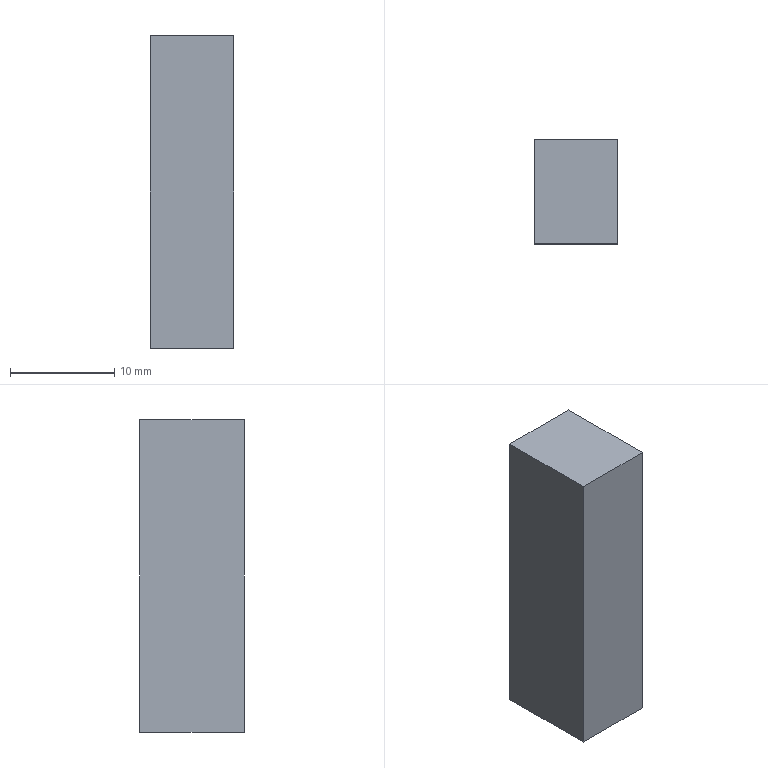Part | SolidWorks | features Extrusion 1 | 1 solid | 6 faces | box 8 x 10 x 30 mm | volume 2400 mm3 | plane 6
STEP:
#1=CARTESIAN_POINT('',(4.,0.,15.));
#2=VERTEX_POINT('',#1);
#3=CARTESIAN_POINT('',(4.,0.,-15.));
#4=VERTEX_POINT('',#3);
#5=CARTESIAN_POINT('',(4.,0.,-15.));
#6=DIRECTION('',(0.,0.,-1.));
#7=VECTOR('',#6,1000.);
#8=LINE('',#5,#7);
#9=EDGE_CURVE('',#2,#4,#8,.T.);
#10=ORIENTED_EDGE('',*,*,#9,.T.);
#11=CARTESIAN_POINT('',(4.,10.,-15.));
#12=VERTEX_POINT('',#11);
#13=CARTESIAN_POINT('',(4.,10.,-15.));
#14=DIRECTION('',(0.,-1.,0.));
#15=VECTOR('',#14,1000.);
#16=LINE('',#13,#15);
#17=EDGE_CURVE('',#12,#4,#16,.T.);
#18=ORIENTED_EDGE('',*,*,#17,.F.);
#19=CARTESIAN_POINT('',(4.,10.,15.));
#20=VERTEX_POINT('',#19);
#21=CARTESIAN_POINT('',(4.,10.,-15.));
#22=DIRECTION('',(0.,0.,-1.));
#23=VECTOR('',#22,1000.);
#24=LINE('',#21,#23);
#25=EDGE_CURVE('',#20,#12,#24,.T.);
#26=ORIENTED_EDGE('',*,*,#25,.F.);
#27=CARTESIAN_POINT('',(4.,10.,15.));
#28=DIRECTION('',(0.,-1.,0.));
#29=VECTOR('',#28,1000.);
#30=LINE('',#27,#29);
#31=EDGE_CURVE('',#20,#2,#30,.T.);
#32=ORIENTED_EDGE('',*,*,#31,.T.);
#33=EDGE_LOOP('',(#10,#18,#26,#32));
#34=FACE_OUTER_BOUND('',#33,.T.);
#35=CARTESIAN_POINT('',(4.,10.,-15.));
#36=DIRECTION('',(-1.,0.,0.));
#37=DIRECTION('',(0.,0.,1.));
#38=AXIS2_PLACEMENT_3D('',#35,#36,#37);
#39=PLANE('',#38);
#40=ADVANCED_FACE('',(#34),#39,.F.);
#41=CARTESIAN_POINT('',(-4.,0.,-15.));
#42=VERTEX_POINT('',#41);
#43=CARTESIAN_POINT('',(-4.,0.,-15.));
#44=DIRECTION('',(-1.,0.,0.));
#45=VECTOR('',#44,1000.);
#46=LINE('',#43,#45);
#47=EDGE_CURVE('',#4,#42,#46,.T.);
#48=ORIENTED_EDGE('',*,*,#47,.T.);
#49=CARTESIAN_POINT('',(-4.,10.,-15.));
#50=VERTEX_POINT('',#49);
#51=CARTESIAN_POINT('',(-4.,10.,-15.));
#52=DIRECTION('',(0.,-1.,0.));
#53=VECTOR('',#52,1000.);
#54=LINE('',#51,#53);
#55=EDGE_CURVE('',#50,#42,#54,.T.);
#56=ORIENTED_EDGE('',*,*,#55,.F.);
#57=CARTESIAN_POINT('',(-4.,10.,-15.));
#58=DIRECTION('',(-1.,0.,0.));
#59=VECTOR('',#58,1000.);
#60=LINE('',#57,#59);
#61=EDGE_CURVE('',#12,#50,#60,.T.);
#62=ORIENTED_EDGE('',*,*,#61,.F.);
#63=ORIENTED_EDGE('',*,*,#17,.T.);
#64=EDGE_LOOP('',(#48,#56,#62,#63));
#65=FACE_OUTER_BOUND('',#64,.T.);
#66=CARTESIAN_POINT('',(-4.,10.,-15.));
#67=DIRECTION('',(0.,0.,1.));
#68=DIRECTION('',(1.,0.,0.));
#69=AXIS2_PLACEMENT_3D('',#66,#67,#68);
#70=PLANE('',#69);
#71=ADVANCED_FACE('',(#65),#70,.F.);
#72=CARTESIAN_POINT('',(-4.,0.,15.));
#73=VERTEX_POINT('',#72);
#74=CARTESIAN_POINT('',(-4.,0.,-15.));
#75=DIRECTION('',(0.,0.,1.));
#76=VECTOR('',#75,1000.);
#77=LINE('',#74,#76);
#78=EDGE_CURVE('',#42,#73,#77,.T.);
#79=ORIENTED_EDGE('',*,*,#78,.T.);
#80=CARTESIAN_POINT('',(-4.,10.,15.));
#81=VERTEX_POINT('',#80);
#82=CARTESIAN_POINT('',(-4.,10.,15.));
#83=DIRECTION('',(0.,-1.,0.));
#84=VECTOR('',#83,1000.);
#85=LINE('',#82,#84);
#86=EDGE_CURVE('',#81,#73,#85,.T.);
#87=ORIENTED_EDGE('',*,*,#86,.F.);
#88=CARTESIAN_POINT('',(-4.,10.,-15.));
#89=DIRECTION('',(0.,0.,1.));
#90=VECTOR('',#89,1000.);
#91=LINE('',#88,#90);
#92=EDGE_CURVE('',#50,#81,#91,.T.);
#93=ORIENTED_EDGE('',*,*,#92,.F.);
#94=ORIENTED_EDGE('',*,*,#55,.T.);
#95=EDGE_LOOP('',(#79,#87,#93,#94));
#96=FACE_OUTER_BOUND('',#95,.T.);
#97=CARTESIAN_POINT('',(-4.,10.,-15.));
#98=DIRECTION('',(1.,0.,0.));
#99=DIRECTION('',(0.,0.,-1.));
#100=AXIS2_PLACEMENT_3D('',#97,#98,#99);
#101=PLANE('',#100);
#102=ADVANCED_FACE('',(#96),#101,.F.);
#103=CARTESIAN_POINT('',(-4.,0.,15.));
#104=DIRECTION('',(1.,0.,0.));
#105=VECTOR('',#104,1000.);
#106=LINE('',#103,#105);
#107=EDGE_CURVE('',#73,#2,#106,.T.);
#108=ORIENTED_EDGE('',*,*,#107,.T.);
#109=ORIENTED_EDGE('',*,*,#31,.F.);
#110=CARTESIAN_POINT('',(-4.,10.,15.));
#111=DIRECTION('',(1.,0.,0.));
#112=VECTOR('',#111,1000.);
#113=LINE('',#110,#112);
#114=EDGE_CURVE('',#81,#20,#113,.T.);
#115=ORIENTED_EDGE('',*,*,#114,.F.);
#116=ORIENTED_EDGE('',*,*,#86,.T.);
#117=EDGE_LOOP('',(#108,#109,#115,#116));
#118=FACE_OUTER_BOUND('',#117,.T.);
#119=CARTESIAN_POINT('',(-4.,10.,15.));
#120=DIRECTION('',(0.,0.,-1.));
#121=DIRECTION('',(-1.,0.,0.));
#122=AXIS2_PLACEMENT_3D('',#119,#120,#121);
#123=PLANE('',#122);
#124=ADVANCED_FACE('',(#118),#123,.F.);
#125=ORIENTED_EDGE('',*,*,#25,.T.);
#126=ORIENTED_EDGE('',*,*,#61,.T.);
#127=ORIENTED_EDGE('',*,*,#92,.T.);
#128=ORIENTED_EDGE('',*,*,#114,.T.);
#129=EDGE_LOOP('',(#125,#126,#127,#128));
#130=FACE_OUTER_BOUND('',#129,.T.);
#131=CARTESIAN_POINT('',(0.,10.,0.));
#132=DIRECTION('',(0.,1.,0.));
#133=DIRECTION('',(0.,0.,1.));
#134=AXIS2_PLACEMENT_3D('',#131,#132,#133);
#135=PLANE('',#134);
#136=ADVANCED_FACE('',(#130),#135,.T.);
#137=ORIENTED_EDGE('',*,*,#9,.F.);
#138=ORIENTED_EDGE('',*,*,#107,.F.);
#139=ORIENTED_EDGE('',*,*,#78,.F.);
#140=ORIENTED_EDGE('',*,*,#47,.F.);
#141=EDGE_LOOP('',(#137,#138,#139,#140));
#142=FACE_OUTER_BOUND('',#141,.T.);
#143=CARTESIAN_POINT('',(0.,0.,0.));
#144=DIRECTION('',(0.,1.,0.));
#145=DIRECTION('',(0.,0.,1.));
#146=AXIS2_PLACEMENT_3D('',#143,#144,#145);
#147=PLANE('',#146);
#148=ADVANCED_FACE('',(#142),#147,.F.);
#149=CLOSED_SHELL('',(#40,#71,#102,#124,#136,#148));
#150=MANIFOLD_SOLID_BREP('',#149);
#151=CARTESIAN_POINT('',(0.,0.,0.));
#152=DIRECTION('',(0.,0.,1.));
#153=DIRECTION('',(1.,0.,0.));
#154=AXIS2_PLACEMENT_3D('',#151,#152,#153);
#155=(LENGTH_UNIT()NAMED_UNIT(*)SI_UNIT(.MILLI.,.METRE.));
#156=UNCERTAINTY_MEASURE_WITH_UNIT(LENGTH_MEASURE(0.00001),#155,'','');
#157=(NAMED_UNIT(*)PLANE_ANGLE_UNIT()SI_UNIT($,.RADIAN.));
#158=(NAMED_UNIT(*)SI_UNIT($,.STERADIAN.)SOLID_ANGLE_UNIT());
#159=(GEOMETRIC_REPRESENTATION_CONTEXT(3)GLOBAL_UNCERTAINTY_ASSIGNED_CONTEXT((#156))GLOBAL_UNIT_ASSIGNED_CONTEXT((#155,#157,#158))REPRESENTATION_CONTEXT('',''));
#160=ADVANCED_BREP_SHAPE_REPRESENTATION('',(#150,#154),#159);